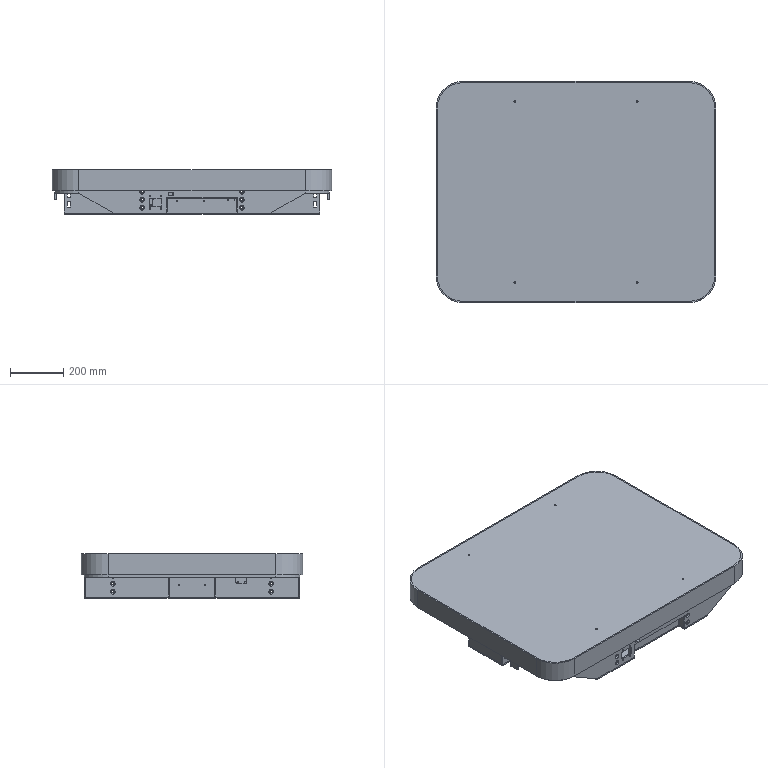Part | NX | features BREP 29 | 42 solids | 763 faces | box 1050 x 830 x 168 mm | volume 13397029 mm3 | plane 422 | cylinder 293 | cone 48 | commonest cylinder face diameters 4 x36 10 x35 6.5 x28 9 x28 2.5 x24 3.4 x22